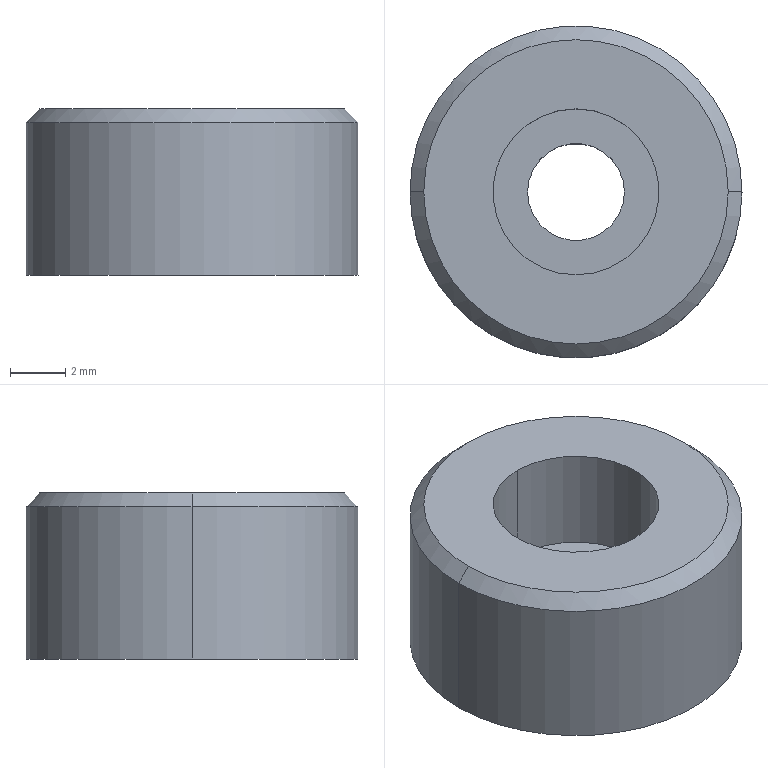Part | NX | features BREP 1 | 1 solid | 11 faces | box 12 x 12 x 6 mm | volume 545.394 mm3 | cylinder 6 | plane 3 | cone 2 | commonest cylinder face diameters 3.5 x2 6 x2 12 x2
STEP:
#1=CARTESIAN_POINT('',(6.,0.,0.));
#2=VERTEX_POINT('',#1);
#3=CARTESIAN_POINT('',(-6.,0.,0.));
#4=VERTEX_POINT('',#3);
#5=CARTESIAN_POINT('',(0.,0.,0.));
#6=DIRECTION('',(0.,0.,1.));
#7=DIRECTION('',(1.,0.,0.));
#8=AXIS2_PLACEMENT_3D('',#5,#6,#7);
#9=CIRCLE('',#8,6.);
#10=EDGE_CURVE('',#2,#4,#9,.T.);
#11=ORIENTED_EDGE('',*,*,#10,.T.);
#12=CARTESIAN_POINT('',(-6.,0.,5.5));
#13=VERTEX_POINT('',#12);
#14=CARTESIAN_POINT('',(-6.,0.,0.));
#15=DIRECTION('',(0.,0.,1.));
#16=VECTOR('',#15,1000.);
#17=LINE('',#14,#16);
#18=EDGE_CURVE('',#13,#4,#17,.F.);
#19=ORIENTED_EDGE('',*,*,#18,.F.);
#20=CARTESIAN_POINT('',(6.,0.,5.5));
#21=VERTEX_POINT('',#20);
#22=CARTESIAN_POINT('',(0.,0.,5.5));
#23=DIRECTION('',(0.,0.,-1.));
#24=DIRECTION('',(1.,0.,0.));
#25=AXIS2_PLACEMENT_3D('',#22,#23,#24);
#26=CIRCLE('',#25,6.);
#27=EDGE_CURVE('',#13,#21,#26,.T.);
#28=ORIENTED_EDGE('',*,*,#27,.T.);
#29=CARTESIAN_POINT('',(6.,0.,0.));
#30=DIRECTION('',(0.,0.,1.));
#31=VECTOR('',#30,1000.);
#32=LINE('',#29,#31);
#33=EDGE_CURVE('',#21,#2,#32,.F.);
#34=ORIENTED_EDGE('',*,*,#33,.T.);
#35=EDGE_LOOP('',(#11,#19,#28,#34));
#36=FACE_BOUND('',#35,.T.);
#37=CARTESIAN_POINT('',(0.,0.,0.));
#38=DIRECTION('',(0.,0.,1.));
#39=DIRECTION('',(1.,0.,0.));
#40=AXIS2_PLACEMENT_3D('',#37,#38,#39);
#41=CYLINDRICAL_SURFACE('',#40,6.);
#42=ADVANCED_FACE('',(#36),#41,.T.);
#43=CARTESIAN_POINT('',(-5.5,0.,6.));
#44=VERTEX_POINT('',#43);
#45=CARTESIAN_POINT('',(5.5,0.,6.));
#46=VERTEX_POINT('',#45);
#47=CARTESIAN_POINT('',(0.,0.,6.));
#48=DIRECTION('',(0.,0.,-1.));
#49=DIRECTION('',(-1.,0.,0.));
#50=AXIS2_PLACEMENT_3D('',#47,#48,#49);
#51=CIRCLE('',#50,5.5);
#52=EDGE_CURVE('',#44,#46,#51,.T.);
#53=ORIENTED_EDGE('',*,*,#52,.T.);
#54=CARTESIAN_POINT('',(6.,0.,5.5));
#55=DIRECTION('',(0.7071,0.,-0.7071));
#56=VECTOR('',#55,1000.);
#57=LINE('',#54,#56);
#58=EDGE_CURVE('',#46,#21,#57,.T.);
#59=ORIENTED_EDGE('',*,*,#58,.T.);
#60=ORIENTED_EDGE('',*,*,#27,.F.);
#61=CARTESIAN_POINT('',(-6.,0.,5.5));
#62=DIRECTION('',(-0.7071,0.,-0.7071));
#63=VECTOR('',#62,1000.);
#64=LINE('',#61,#63);
#65=EDGE_CURVE('',#44,#13,#64,.T.);
#66=ORIENTED_EDGE('',*,*,#65,.F.);
#67=EDGE_LOOP('',(#53,#59,#60,#66));
#68=FACE_BOUND('',#67,.T.);
#69=CARTESIAN_POINT('',(0.,0.,5.5));
#70=DIRECTION('',(0.,0.,-1.));
#71=DIRECTION('',(-1.,0.,0.));
#72=AXIS2_PLACEMENT_3D('',#69,#70,#71);
#73=CONICAL_SURFACE('',#72,6.,0.7854);
#74=ADVANCED_FACE('',(#68),#73,.T.);
#75=CARTESIAN_POINT('',(1.75,0.,2.2));
#76=VERTEX_POINT('',#75);
#77=CARTESIAN_POINT('',(-1.75,0.,2.2));
#78=VERTEX_POINT('',#77);
#79=CARTESIAN_POINT('',(0.,0.,2.2));
#80=DIRECTION('',(0.,0.,-1.));
#81=DIRECTION('',(-1.,0.,0.));
#82=AXIS2_PLACEMENT_3D('',#79,#80,#81);
#83=CIRCLE('',#82,1.75);
#84=EDGE_CURVE('',#76,#78,#83,.T.);
#85=ORIENTED_EDGE('',*,*,#84,.F.);
#86=CARTESIAN_POINT('',(1.75,0.,0.));
#87=VERTEX_POINT('',#86);
#88=CARTESIAN_POINT('',(1.75,0.,2.2));
#89=DIRECTION('',(0.,0.,-1.));
#90=VECTOR('',#89,1000.);
#91=LINE('',#88,#90);
#92=EDGE_CURVE('',#76,#87,#91,.T.);
#93=ORIENTED_EDGE('',*,*,#92,.T.);
#94=CARTESIAN_POINT('',(-1.75,0.,0.));
#95=VERTEX_POINT('',#94);
#96=CARTESIAN_POINT('',(0.,0.,0.));
#97=DIRECTION('',(0.,0.,1.));
#98=DIRECTION('',(-1.,0.,0.));
#99=AXIS2_PLACEMENT_3D('',#96,#97,#98);
#100=CIRCLE('',#99,1.75);
#101=EDGE_CURVE('',#95,#87,#100,.T.);
#102=ORIENTED_EDGE('',*,*,#101,.F.);
#103=CARTESIAN_POINT('',(-1.75,0.,2.2));
#104=DIRECTION('',(0.,0.,-1.));
#105=VECTOR('',#104,1000.);
#106=LINE('',#103,#105);
#107=EDGE_CURVE('',#78,#95,#106,.T.);
#108=ORIENTED_EDGE('',*,*,#107,.F.);
#109=EDGE_LOOP('',(#85,#93,#102,#108));
#110=FACE_BOUND('',#109,.T.);
#111=CARTESIAN_POINT('',(0.,0.,2.2));
#112=DIRECTION('',(0.,0.,-1.));
#113=DIRECTION('',(-1.,0.,0.));
#114=AXIS2_PLACEMENT_3D('',#111,#112,#113);
#115=CYLINDRICAL_SURFACE('',#114,1.75);
#116=ADVANCED_FACE('',(#110),#115,.F.);
#117=CARTESIAN_POINT('',(0.,3.,6.));
#118=VERTEX_POINT('',#117);
#119=CARTESIAN_POINT('',(0.,-3.,6.));
#120=VERTEX_POINT('',#119);
#121=CARTESIAN_POINT('',(0.,0.,6.));
#122=DIRECTION('',(0.,0.,1.));
#123=DIRECTION('',(0.,1.,0.));
#124=AXIS2_PLACEMENT_3D('',#121,#122,#123);
#125=CIRCLE('',#124,3.);
#126=EDGE_CURVE('',#118,#120,#125,.T.);
#127=ORIENTED_EDGE('',*,*,#126,.T.);
#128=CARTESIAN_POINT('',(0.,-3.,2.2));
#129=VERTEX_POINT('',#128);
#130=CARTESIAN_POINT('',(0.,-3.,6.));
#131=DIRECTION('',(0.,0.,-1.));
#132=VECTOR('',#131,1000.);
#133=LINE('',#130,#132);
#134=EDGE_CURVE('',#129,#120,#133,.F.);
#135=ORIENTED_EDGE('',*,*,#134,.F.);
#136=CARTESIAN_POINT('',(0.,3.,2.2));
#137=VERTEX_POINT('',#136);
#138=CARTESIAN_POINT('',(0.,0.,2.2));
#139=DIRECTION('',(0.,0.,1.));
#140=DIRECTION('',(0.,1.,0.));
#141=AXIS2_PLACEMENT_3D('',#138,#139,#140);
#142=CIRCLE('',#141,3.);
#143=EDGE_CURVE('',#137,#129,#142,.T.);
#144=ORIENTED_EDGE('',*,*,#143,.F.);
#145=CARTESIAN_POINT('',(0.,3.,6.));
#146=DIRECTION('',(0.,0.,-1.));
#147=VECTOR('',#146,1000.);
#148=LINE('',#145,#147);
#149=EDGE_CURVE('',#137,#118,#148,.F.);
#150=ORIENTED_EDGE('',*,*,#149,.T.);
#151=EDGE_LOOP('',(#127,#135,#144,#150));
#152=FACE_BOUND('',#151,.T.);
#153=CARTESIAN_POINT('',(0.,0.,6.));
#154=DIRECTION('',(0.,0.,-1.));
#155=DIRECTION('',(0.,1.,0.));
#156=AXIS2_PLACEMENT_3D('',#153,#154,#155);
#157=CYLINDRICAL_SURFACE('',#156,3.);
#158=ADVANCED_FACE('',(#152),#157,.F.);
#159=ORIENTED_EDGE('',*,*,#18,.T.);
#160=CARTESIAN_POINT('',(0.,0.,0.));
#161=DIRECTION('',(0.,0.,1.));
#162=DIRECTION('',(1.,0.,0.));
#163=AXIS2_PLACEMENT_3D('',#160,#161,#162);
#164=CIRCLE('',#163,6.);
#165=EDGE_CURVE('',#4,#2,#164,.T.);
#166=ORIENTED_EDGE('',*,*,#165,.T.);
#167=ORIENTED_EDGE('',*,*,#33,.F.);
#168=CARTESIAN_POINT('',(0.,0.,5.5));
#169=DIRECTION('',(0.,0.,-1.));
#170=DIRECTION('',(1.,0.,0.));
#171=AXIS2_PLACEMENT_3D('',#168,#169,#170);
#172=CIRCLE('',#171,6.);
#173=EDGE_CURVE('',#21,#13,#172,.T.);
#174=ORIENTED_EDGE('',*,*,#173,.T.);
#175=EDGE_LOOP('',(#159,#166,#167,#174));
#176=FACE_BOUND('',#175,.T.);
#177=CARTESIAN_POINT('',(0.,0.,0.));
#178=DIRECTION('',(0.,0.,1.));
#179=DIRECTION('',(1.,0.,0.));
#180=AXIS2_PLACEMENT_3D('',#177,#178,#179);
#181=CYLINDRICAL_SURFACE('',#180,6.);
#182=ADVANCED_FACE('',(#176),#181,.T.);
#183=ORIENTED_EDGE('',*,*,#58,.F.);
#184=CARTESIAN_POINT('',(0.,0.,6.));
#185=DIRECTION('',(0.,0.,-1.));
#186=DIRECTION('',(-1.,0.,0.));
#187=AXIS2_PLACEMENT_3D('',#184,#185,#186);
#188=CIRCLE('',#187,5.5);
#189=EDGE_CURVE('',#46,#44,#188,.T.);
#190=ORIENTED_EDGE('',*,*,#189,.T.);
#191=ORIENTED_EDGE('',*,*,#65,.T.);
#192=ORIENTED_EDGE('',*,*,#173,.F.);
#193=EDGE_LOOP('',(#183,#190,#191,#192));
#194=FACE_BOUND('',#193,.T.);
#195=CARTESIAN_POINT('',(0.,0.,5.5));
#196=DIRECTION('',(0.,0.,-1.));
#197=DIRECTION('',(-1.,0.,0.));
#198=AXIS2_PLACEMENT_3D('',#195,#196,#197);
#199=CONICAL_SURFACE('',#198,6.,0.7854);
#200=ADVANCED_FACE('',(#194),#199,.T.);
#201=ORIENTED_EDGE('',*,*,#10,.F.);
#202=ORIENTED_EDGE('',*,*,#165,.F.);
#203=EDGE_LOOP('',(#201,#202));
#204=FACE_BOUND('',#203,.T.);
#205=ORIENTED_EDGE('',*,*,#101,.T.);
#206=CARTESIAN_POINT('',(0.,0.,0.));
#207=DIRECTION('',(0.,0.,1.));
#208=DIRECTION('',(-1.,0.,0.));
#209=AXIS2_PLACEMENT_3D('',#206,#207,#208);
#210=CIRCLE('',#209,1.75);
#211=EDGE_CURVE('',#87,#95,#210,.T.);
#212=ORIENTED_EDGE('',*,*,#211,.T.);
#213=EDGE_LOOP('',(#205,#212));
#214=FACE_BOUND('',#213,.T.);
#215=CARTESIAN_POINT('',(0.,0.,0.));
#216=DIRECTION('',(0.,0.,-1.));
#217=DIRECTION('',(0.,-1.,0.));
#218=AXIS2_PLACEMENT_3D('',#215,#216,#217);
#219=PLANE('',#218);
#220=ADVANCED_FACE('',(#204,#214),#219,.T.);
#221=ORIENTED_EDGE('',*,*,#52,.F.);
#222=ORIENTED_EDGE('',*,*,#189,.F.);
#223=EDGE_LOOP('',(#221,#222));
#224=FACE_BOUND('',#223,.T.);
#225=ORIENTED_EDGE('',*,*,#126,.F.);
#226=CARTESIAN_POINT('',(0.,0.,6.));
#227=DIRECTION('',(0.,0.,1.));
#228=DIRECTION('',(0.,1.,0.));
#229=AXIS2_PLACEMENT_3D('',#226,#227,#228);
#230=CIRCLE('',#229,3.);
#231=EDGE_CURVE('',#120,#118,#230,.T.);
#232=ORIENTED_EDGE('',*,*,#231,.F.);
#233=EDGE_LOOP('',(#225,#232));
#234=FACE_BOUND('',#233,.T.);
#235=CARTESIAN_POINT('',(0.,0.,6.));
#236=DIRECTION('',(0.,0.,-1.));
#237=DIRECTION('',(0.,-1.,0.));
#238=AXIS2_PLACEMENT_3D('',#235,#236,#237);
#239=PLANE('',#238);
#240=ADVANCED_FACE('',(#224,#234),#239,.F.);
#241=ORIENTED_EDGE('',*,*,#92,.F.);
#242=CARTESIAN_POINT('',(0.,0.,2.2));
#243=DIRECTION('',(0.,0.,-1.));
#244=DIRECTION('',(-1.,0.,0.));
#245=AXIS2_PLACEMENT_3D('',#242,#243,#244);
#246=CIRCLE('',#245,1.75);
#247=EDGE_CURVE('',#78,#76,#246,.T.);
#248=ORIENTED_EDGE('',*,*,#247,.F.);
#249=ORIENTED_EDGE('',*,*,#107,.T.);
#250=ORIENTED_EDGE('',*,*,#211,.F.);
#251=EDGE_LOOP('',(#241,#248,#249,#250));
#252=FACE_BOUND('',#251,.T.);
#253=CARTESIAN_POINT('',(0.,0.,2.2));
#254=DIRECTION('',(0.,0.,-1.));
#255=DIRECTION('',(-1.,0.,0.));
#256=AXIS2_PLACEMENT_3D('',#253,#254,#255);
#257=CYLINDRICAL_SURFACE('',#256,1.75);
#258=ADVANCED_FACE('',(#252),#257,.F.);
#259=ORIENTED_EDGE('',*,*,#134,.T.);
#260=ORIENTED_EDGE('',*,*,#231,.T.);
#261=ORIENTED_EDGE('',*,*,#149,.F.);
#262=CARTESIAN_POINT('',(0.,0.,2.2));
#263=DIRECTION('',(0.,0.,1.));
#264=DIRECTION('',(0.,1.,0.));
#265=AXIS2_PLACEMENT_3D('',#262,#263,#264);
#266=CIRCLE('',#265,3.);
#267=EDGE_CURVE('',#129,#137,#266,.T.);
#268=ORIENTED_EDGE('',*,*,#267,.F.);
#269=EDGE_LOOP('',(#259,#260,#261,#268));
#270=FACE_BOUND('',#269,.T.);
#271=CARTESIAN_POINT('',(0.,0.,6.));
#272=DIRECTION('',(0.,0.,-1.));
#273=DIRECTION('',(0.,1.,0.));
#274=AXIS2_PLACEMENT_3D('',#271,#272,#273);
#275=CYLINDRICAL_SURFACE('',#274,3.);
#276=ADVANCED_FACE('',(#270),#275,.F.);
#277=ORIENTED_EDGE('',*,*,#143,.T.);
#278=ORIENTED_EDGE('',*,*,#267,.T.);
#279=EDGE_LOOP('',(#277,#278));
#280=FACE_BOUND('',#279,.T.);
#281=ORIENTED_EDGE('',*,*,#247,.T.);
#282=ORIENTED_EDGE('',*,*,#84,.T.);
#283=EDGE_LOOP('',(#281,#282));
#284=FACE_BOUND('',#283,.T.);
#285=CARTESIAN_POINT('',(-3.,3.06,2.2));
#286=DIRECTION('',(0.,0.,-1.));
#287=DIRECTION('',(0.,-1.,0.));
#288=AXIS2_PLACEMENT_3D('',#285,#286,#287);
#289=PLANE('',#288);
#290=ADVANCED_FACE('',(#280,#284),#289,.F.);
#291=CLOSED_SHELL('',(#42,#74,#116,#158,#182,#200,#220,#240,#258,#276,#290));
#292=MANIFOLD_SOLID_BREP('',#291);
#293=(LENGTH_UNIT()NAMED_UNIT(*)SI_UNIT(.MILLI.,.METRE.));
#294=UNCERTAINTY_MEASURE_WITH_UNIT(LENGTH_MEASURE(0.00001),#293,'','');
#295=(NAMED_UNIT(*)PLANE_ANGLE_UNIT()SI_UNIT($,.RADIAN.));
#296=(NAMED_UNIT(*)SI_UNIT($,.STERADIAN.)SOLID_ANGLE_UNIT());
#297=(GEOMETRIC_REPRESENTATION_CONTEXT(3)GLOBAL_UNCERTAINTY_ASSIGNED_CONTEXT((#294))GLOBAL_UNIT_ASSIGNED_CONTEXT((#293,#295,#296))REPRESENTATION_CONTEXT('',''));
#298=ADVANCED_BREP_SHAPE_REPRESENTATION('',(#292),#297);